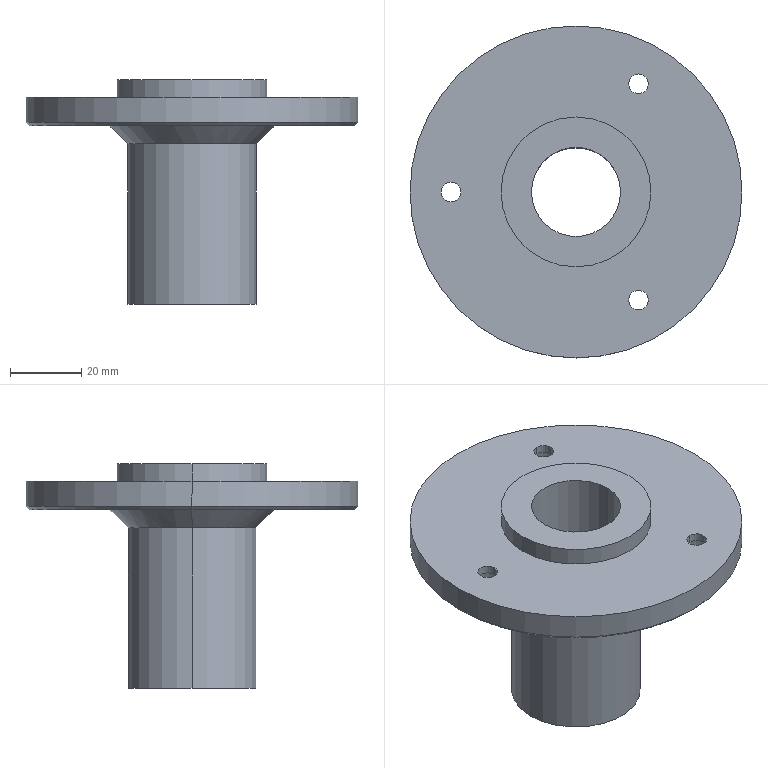Part | STEP file | PN_0026 Snap-ring connector | 1 solid | 34 faces | box 93 x 93 x 63 mm | volume 79836 mm3 | cylinder 22 | plane 8 | cone 4 | commonest cylinder face diameters 5.5 x6 10 x6 25 x2 30 x2 36 x2 42 x2